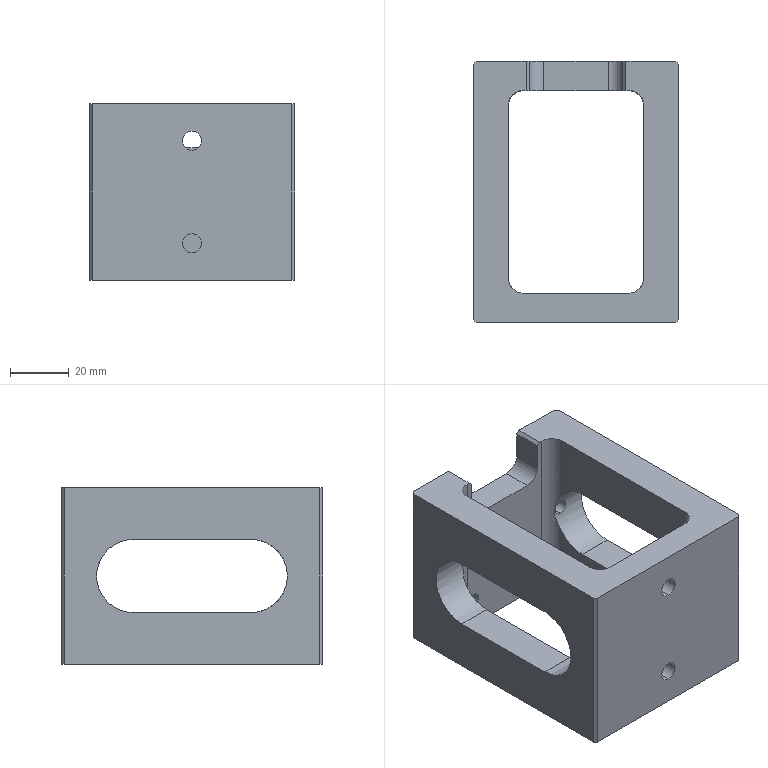Part | SolidWorks | features HoleWzd 4, Fillet 2, ICE 2, Chamfer 1, Extrusion 1 | 1 solid | 53 faces | box 70 x 89 x 60 mm | volume 142318 mm3 | plane 25 | cylinder 24 | cone 4 | commonest cylinder face diameters 10 x6 25 x6 5 x4 6 x4 6.5 x4